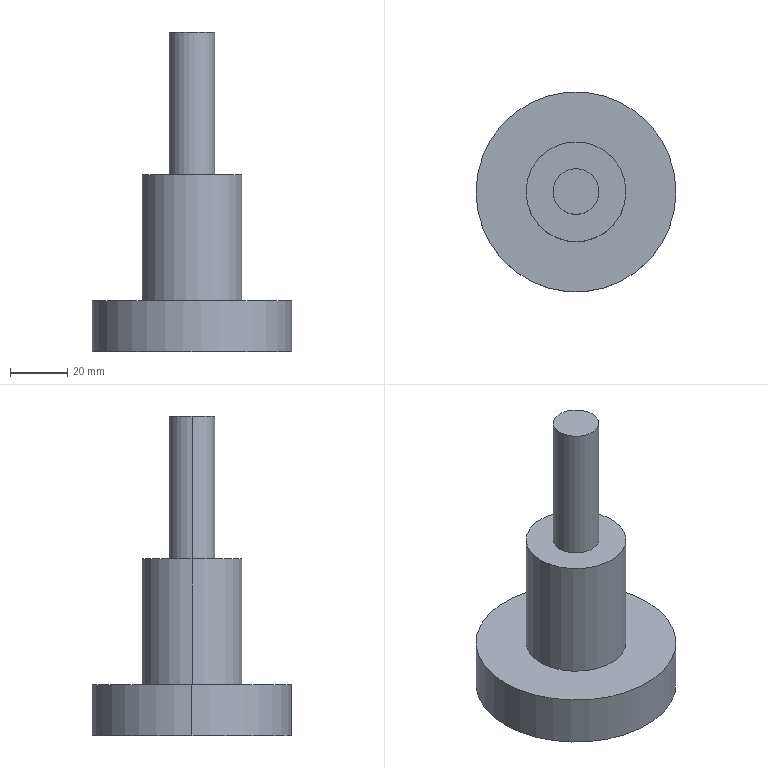Part | SolidWorks | features Revolution 1 | 1 solid | 10 faces | box 70 x 70 x 112 mm | volume 121658 mm3 | cylinder 6 | plane 4 | commonest cylinder face diameters 16 x2 35 x2 70 x2
STEP:
#1=CARTESIAN_POINT('',(35.,0.,-112.));
#2=VERTEX_POINT('',#1);
#3=CARTESIAN_POINT('',(-35.,0.,-112.));
#4=VERTEX_POINT('',#3);
#5=CARTESIAN_POINT('',(0.,0.,-112.));
#6=DIRECTION('',(0.,0.,1.));
#7=DIRECTION('',(1.,0.,0.));
#8=AXIS2_PLACEMENT_3D('',#5,#6,#7);
#9=CIRCLE('',#8,35.);
#10=EDGE_CURVE('',#2,#4,#9,.T.);
#11=ORIENTED_EDGE('',*,*,#10,.T.);
#12=CARTESIAN_POINT('',(-35.,0.,-94.));
#13=VERTEX_POINT('',#12);
#14=CARTESIAN_POINT('',(-35.,0.,0.));
#15=DIRECTION('',(0.,0.,1.));
#16=VECTOR('',#15,1000.);
#17=LINE('',#14,#16);
#18=EDGE_CURVE('',#4,#13,#17,.T.);
#19=ORIENTED_EDGE('',*,*,#18,.T.);
#20=CARTESIAN_POINT('',(35.,0.,-94.));
#21=VERTEX_POINT('',#20);
#22=CARTESIAN_POINT('',(0.,0.,-94.));
#23=DIRECTION('',(0.,0.,1.));
#24=DIRECTION('',(1.,0.,0.));
#25=AXIS2_PLACEMENT_3D('',#22,#23,#24);
#26=CIRCLE('',#25,35.);
#27=EDGE_CURVE('',#21,#13,#26,.T.);
#28=ORIENTED_EDGE('',*,*,#27,.F.);
#29=CARTESIAN_POINT('',(35.,0.,0.));
#30=DIRECTION('',(0.,0.,1.));
#31=VECTOR('',#30,1000.);
#32=LINE('',#29,#31);
#33=EDGE_CURVE('',#2,#21,#32,.T.);
#34=ORIENTED_EDGE('',*,*,#33,.F.);
#35=EDGE_LOOP('',(#11,#19,#28,#34));
#36=FACE_OUTER_BOUND('',#35,.T.);
#37=CARTESIAN_POINT('',(0.,0.,0.));
#38=DIRECTION('',(0.,0.,1.));
#39=DIRECTION('',(1.,0.,0.));
#40=AXIS2_PLACEMENT_3D('',#37,#38,#39);
#41=CYLINDRICAL_SURFACE('',#40,35.);
#42=ADVANCED_FACE('',(#36),#41,.T.);
#43=CARTESIAN_POINT('',(8.,0.,-50.));
#44=VERTEX_POINT('',#43);
#45=CARTESIAN_POINT('',(-8.,0.,-50.));
#46=VERTEX_POINT('',#45);
#47=CARTESIAN_POINT('',(0.,0.,-50.));
#48=DIRECTION('',(0.,0.,1.));
#49=DIRECTION('',(1.,0.,0.));
#50=AXIS2_PLACEMENT_3D('',#47,#48,#49);
#51=CIRCLE('',#50,8.);
#52=EDGE_CURVE('',#44,#46,#51,.T.);
#53=ORIENTED_EDGE('',*,*,#52,.T.);
#54=CARTESIAN_POINT('',(-8.,0.,0.));
#55=VERTEX_POINT('',#54);
#56=CARTESIAN_POINT('',(-8.,0.,0.));
#57=DIRECTION('',(0.,0.,1.));
#58=VECTOR('',#57,1000.);
#59=LINE('',#56,#58);
#60=EDGE_CURVE('',#46,#55,#59,.T.);
#61=ORIENTED_EDGE('',*,*,#60,.T.);
#62=CARTESIAN_POINT('',(8.,0.,0.));
#63=VERTEX_POINT('',#62);
#64=CARTESIAN_POINT('',(0.,0.,0.));
#65=DIRECTION('',(0.,0.,1.));
#66=DIRECTION('',(1.,0.,0.));
#67=AXIS2_PLACEMENT_3D('',#64,#65,#66);
#68=CIRCLE('',#67,8.);
#69=EDGE_CURVE('',#63,#55,#68,.T.);
#70=ORIENTED_EDGE('',*,*,#69,.F.);
#71=CARTESIAN_POINT('',(8.,0.,0.));
#72=DIRECTION('',(0.,0.,1.));
#73=VECTOR('',#72,1000.);
#74=LINE('',#71,#73);
#75=EDGE_CURVE('',#44,#63,#74,.T.);
#76=ORIENTED_EDGE('',*,*,#75,.F.);
#77=EDGE_LOOP('',(#53,#61,#70,#76));
#78=FACE_OUTER_BOUND('',#77,.T.);
#79=CARTESIAN_POINT('',(0.,0.,0.));
#80=DIRECTION('',(0.,0.,1.));
#81=DIRECTION('',(1.,0.,0.));
#82=AXIS2_PLACEMENT_3D('',#79,#80,#81);
#83=CYLINDRICAL_SURFACE('',#82,8.);
#84=ADVANCED_FACE('',(#78),#83,.T.);
#85=CARTESIAN_POINT('',(17.5,0.,-94.));
#86=VERTEX_POINT('',#85);
#87=CARTESIAN_POINT('',(-17.5,0.,-94.));
#88=VERTEX_POINT('',#87);
#89=CARTESIAN_POINT('',(0.,0.,-94.));
#90=DIRECTION('',(0.,0.,1.));
#91=DIRECTION('',(1.,0.,0.));
#92=AXIS2_PLACEMENT_3D('',#89,#90,#91);
#93=CIRCLE('',#92,17.5);
#94=EDGE_CURVE('',#86,#88,#93,.T.);
#95=ORIENTED_EDGE('',*,*,#94,.T.);
#96=CARTESIAN_POINT('',(-17.5,0.,-50.));
#97=VERTEX_POINT('',#96);
#98=CARTESIAN_POINT('',(-17.5,0.,0.));
#99=DIRECTION('',(0.,0.,1.));
#100=VECTOR('',#99,1000.);
#101=LINE('',#98,#100);
#102=EDGE_CURVE('',#88,#97,#101,.T.);
#103=ORIENTED_EDGE('',*,*,#102,.T.);
#104=CARTESIAN_POINT('',(17.5,0.,-50.));
#105=VERTEX_POINT('',#104);
#106=CARTESIAN_POINT('',(0.,0.,-50.));
#107=DIRECTION('',(0.,0.,1.));
#108=DIRECTION('',(1.,0.,0.));
#109=AXIS2_PLACEMENT_3D('',#106,#107,#108);
#110=CIRCLE('',#109,17.5);
#111=EDGE_CURVE('',#105,#97,#110,.T.);
#112=ORIENTED_EDGE('',*,*,#111,.F.);
#113=CARTESIAN_POINT('',(17.5,0.,0.));
#114=DIRECTION('',(0.,0.,1.));
#115=VECTOR('',#114,1000.);
#116=LINE('',#113,#115);
#117=EDGE_CURVE('',#86,#105,#116,.T.);
#118=ORIENTED_EDGE('',*,*,#117,.F.);
#119=EDGE_LOOP('',(#95,#103,#112,#118));
#120=FACE_OUTER_BOUND('',#119,.T.);
#121=CARTESIAN_POINT('',(0.,0.,0.));
#122=DIRECTION('',(0.,0.,1.));
#123=DIRECTION('',(1.,0.,0.));
#124=AXIS2_PLACEMENT_3D('',#121,#122,#123);
#125=CYLINDRICAL_SURFACE('',#124,17.5);
#126=ADVANCED_FACE('',(#120),#125,.T.);
#127=ORIENTED_EDGE('',*,*,#94,.F.);
#128=CARTESIAN_POINT('',(0.,0.,-94.));
#129=DIRECTION('',(0.,0.,1.));
#130=DIRECTION('',(1.,0.,0.));
#131=AXIS2_PLACEMENT_3D('',#128,#129,#130);
#132=CIRCLE('',#131,17.5);
#133=EDGE_CURVE('',#88,#86,#132,.T.);
#134=ORIENTED_EDGE('',*,*,#133,.F.);
#135=EDGE_LOOP('',(#127,#134));
#136=FACE_BOUND('',#135,.T.);
#137=ORIENTED_EDGE('',*,*,#27,.T.);
#138=CARTESIAN_POINT('',(0.,0.,-94.));
#139=DIRECTION('',(0.,0.,1.));
#140=DIRECTION('',(1.,0.,0.));
#141=AXIS2_PLACEMENT_3D('',#138,#139,#140);
#142=CIRCLE('',#141,35.);
#143=EDGE_CURVE('',#13,#21,#142,.T.);
#144=ORIENTED_EDGE('',*,*,#143,.T.);
#145=EDGE_LOOP('',(#137,#144));
#146=FACE_OUTER_BOUND('',#145,.T.);
#147=CARTESIAN_POINT('',(0.,0.,-94.));
#148=DIRECTION('',(0.,0.,-1.));
#149=DIRECTION('',(-1.,0.,0.));
#150=AXIS2_PLACEMENT_3D('',#147,#148,#149);
#151=PLANE('',#150);
#152=ADVANCED_FACE('',(#136,#146),#151,.F.);
#153=ORIENTED_EDGE('',*,*,#102,.F.);
#154=ORIENTED_EDGE('',*,*,#133,.T.);
#155=ORIENTED_EDGE('',*,*,#117,.T.);
#156=CARTESIAN_POINT('',(0.,0.,-50.));
#157=DIRECTION('',(0.,0.,1.));
#158=DIRECTION('',(1.,0.,0.));
#159=AXIS2_PLACEMENT_3D('',#156,#157,#158);
#160=CIRCLE('',#159,17.5);
#161=EDGE_CURVE('',#97,#105,#160,.T.);
#162=ORIENTED_EDGE('',*,*,#161,.F.);
#163=EDGE_LOOP('',(#153,#154,#155,#162));
#164=FACE_OUTER_BOUND('',#163,.T.);
#165=CARTESIAN_POINT('',(0.,0.,0.));
#166=DIRECTION('',(0.,0.,1.));
#167=DIRECTION('',(1.,0.,0.));
#168=AXIS2_PLACEMENT_3D('',#165,#166,#167);
#169=CYLINDRICAL_SURFACE('',#168,17.5);
#170=ADVANCED_FACE('',(#164),#169,.T.);
#171=ORIENTED_EDGE('',*,*,#52,.F.);
#172=CARTESIAN_POINT('',(0.,0.,-50.));
#173=DIRECTION('',(0.,0.,1.));
#174=DIRECTION('',(1.,0.,0.));
#175=AXIS2_PLACEMENT_3D('',#172,#173,#174);
#176=CIRCLE('',#175,8.);
#177=EDGE_CURVE('',#46,#44,#176,.T.);
#178=ORIENTED_EDGE('',*,*,#177,.F.);
#179=EDGE_LOOP('',(#171,#178));
#180=FACE_BOUND('',#179,.T.);
#181=ORIENTED_EDGE('',*,*,#111,.T.);
#182=ORIENTED_EDGE('',*,*,#161,.T.);
#183=EDGE_LOOP('',(#181,#182));
#184=FACE_OUTER_BOUND('',#183,.T.);
#185=CARTESIAN_POINT('',(0.,0.,-50.));
#186=DIRECTION('',(0.,0.,-1.));
#187=DIRECTION('',(-1.,0.,0.));
#188=AXIS2_PLACEMENT_3D('',#185,#186,#187);
#189=PLANE('',#188);
#190=ADVANCED_FACE('',(#180,#184),#189,.F.);
#191=ORIENTED_EDGE('',*,*,#60,.F.);
#192=ORIENTED_EDGE('',*,*,#177,.T.);
#193=ORIENTED_EDGE('',*,*,#75,.T.);
#194=CARTESIAN_POINT('',(0.,0.,0.));
#195=DIRECTION('',(0.,0.,1.));
#196=DIRECTION('',(1.,0.,0.));
#197=AXIS2_PLACEMENT_3D('',#194,#195,#196);
#198=CIRCLE('',#197,8.);
#199=EDGE_CURVE('',#55,#63,#198,.T.);
#200=ORIENTED_EDGE('',*,*,#199,.F.);
#201=EDGE_LOOP('',(#191,#192,#193,#200));
#202=FACE_OUTER_BOUND('',#201,.T.);
#203=CARTESIAN_POINT('',(0.,0.,0.));
#204=DIRECTION('',(0.,0.,1.));
#205=DIRECTION('',(1.,0.,0.));
#206=AXIS2_PLACEMENT_3D('',#203,#204,#205);
#207=CYLINDRICAL_SURFACE('',#206,8.);
#208=ADVANCED_FACE('',(#202),#207,.T.);
#209=ORIENTED_EDGE('',*,*,#69,.T.);
#210=ORIENTED_EDGE('',*,*,#199,.T.);
#211=EDGE_LOOP('',(#209,#210));
#212=FACE_OUTER_BOUND('',#211,.T.);
#213=CARTESIAN_POINT('',(0.,0.,0.));
#214=DIRECTION('',(0.,0.,1.));
#215=DIRECTION('',(1.,0.,0.));
#216=AXIS2_PLACEMENT_3D('',#213,#214,#215);
#217=PLANE('',#216);
#218=ADVANCED_FACE('',(#212),#217,.T.);
#219=ORIENTED_EDGE('',*,*,#10,.F.);
#220=CARTESIAN_POINT('',(0.,0.,-112.));
#221=DIRECTION('',(0.,0.,1.));
#222=DIRECTION('',(1.,0.,0.));
#223=AXIS2_PLACEMENT_3D('',#220,#221,#222);
#224=CIRCLE('',#223,35.);
#225=EDGE_CURVE('',#4,#2,#224,.T.);
#226=ORIENTED_EDGE('',*,*,#225,.F.);
#227=EDGE_LOOP('',(#219,#226));
#228=FACE_OUTER_BOUND('',#227,.T.);
#229=CARTESIAN_POINT('',(0.,0.,-112.));
#230=DIRECTION('',(0.,0.,-1.));
#231=DIRECTION('',(-1.,0.,0.));
#232=AXIS2_PLACEMENT_3D('',#229,#230,#231);
#233=PLANE('',#232);
#234=ADVANCED_FACE('',(#228),#233,.T.);
#235=ORIENTED_EDGE('',*,*,#18,.F.);
#236=ORIENTED_EDGE('',*,*,#225,.T.);
#237=ORIENTED_EDGE('',*,*,#33,.T.);
#238=ORIENTED_EDGE('',*,*,#143,.F.);
#239=EDGE_LOOP('',(#235,#236,#237,#238));
#240=FACE_OUTER_BOUND('',#239,.T.);
#241=CARTESIAN_POINT('',(0.,0.,0.));
#242=DIRECTION('',(0.,0.,1.));
#243=DIRECTION('',(1.,0.,0.));
#244=AXIS2_PLACEMENT_3D('',#241,#242,#243);
#245=CYLINDRICAL_SURFACE('',#244,35.);
#246=ADVANCED_FACE('',(#240),#245,.T.);
#247=CLOSED_SHELL('',(#42,#84,#126,#152,#170,#190,#208,#218,#234,#246));
#248=MANIFOLD_SOLID_BREP('',#247);
#249=CARTESIAN_POINT('',(0.,0.,0.));
#250=DIRECTION('',(0.,0.,1.));
#251=DIRECTION('',(1.,0.,0.));
#252=AXIS2_PLACEMENT_3D('',#249,#250,#251);
#253=(LENGTH_UNIT()NAMED_UNIT(*)SI_UNIT(.MILLI.,.METRE.));
#254=UNCERTAINTY_MEASURE_WITH_UNIT(LENGTH_MEASURE(0.00001),#253,'','');
#255=(NAMED_UNIT(*)PLANE_ANGLE_UNIT()SI_UNIT($,.RADIAN.));
#256=(NAMED_UNIT(*)SI_UNIT($,.STERADIAN.)SOLID_ANGLE_UNIT());
#257=(GEOMETRIC_REPRESENTATION_CONTEXT(3)GLOBAL_UNCERTAINTY_ASSIGNED_CONTEXT((#254))GLOBAL_UNIT_ASSIGNED_CONTEXT((#253,#255,#256))REPRESENTATION_CONTEXT('',''));
#258=ADVANCED_BREP_SHAPE_REPRESENTATION('',(#248,#252),#257);